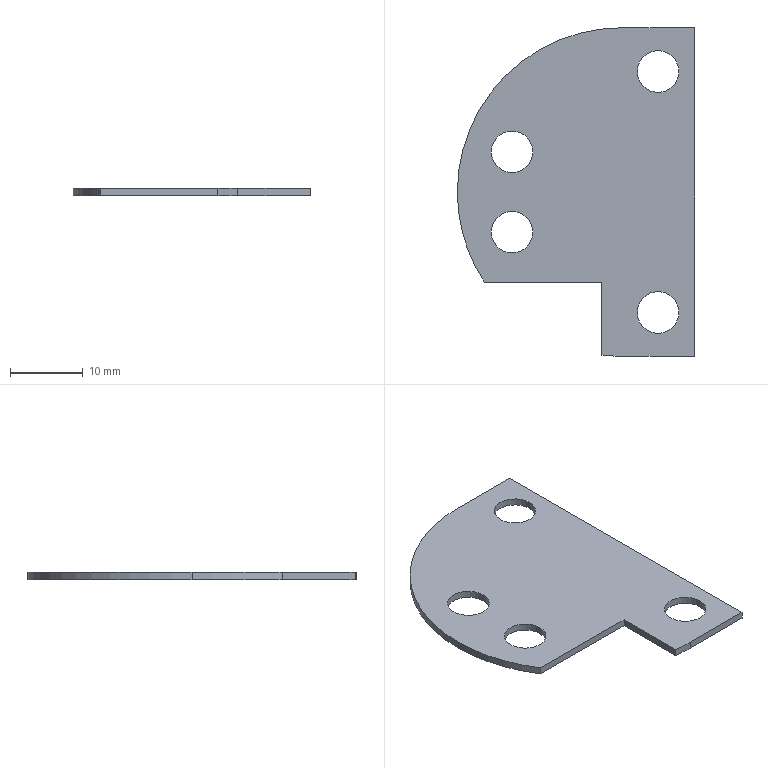Part | SolidWorks | features BaseBody 1, ICE 1 | 1 solid | 18 faces | box 32.5 x 45 x 1 mm | volume 1036 mm3 | cylinder 11 | plane 7 | commonest cylinder face diameters 5.7 x8 45 x3
STEP:
#1=CARTESIAN_POINT('',(-22.85,5.5,1.));
#2=VERTEX_POINT('',#1);
#3=CARTESIAN_POINT('',(-17.15,5.5,1.));
#4=VERTEX_POINT('',#3);
#5=CARTESIAN_POINT('',(-20.,5.5,1.));
#6=DIRECTION('',(0.,0.,1.));
#7=DIRECTION('',(1.,0.,0.));
#8=AXIS2_PLACEMENT_3D('',#5,#6,#7);
#9=CIRCLE('',#8,2.85);
#10=EDGE_CURVE('',#2,#4,#9,.T.);
#11=ORIENTED_EDGE('',*,*,#10,.T.);
#12=CARTESIAN_POINT('',(-17.15,5.5,0.));
#13=VERTEX_POINT('',#12);
#14=CARTESIAN_POINT('',(-17.15,5.5,1.));
#15=DIRECTION('',(0.,0.,-1.));
#16=VECTOR('',#15,1000.);
#17=LINE('',#14,#16);
#18=EDGE_CURVE('',#4,#13,#17,.T.);
#19=ORIENTED_EDGE('',*,*,#18,.T.);
#20=CARTESIAN_POINT('',(-22.85,5.5,0.));
#21=VERTEX_POINT('',#20);
#22=CARTESIAN_POINT('',(-20.,5.5,0.));
#23=DIRECTION('',(0.,0.,1.));
#24=DIRECTION('',(1.,0.,0.));
#25=AXIS2_PLACEMENT_3D('',#22,#23,#24);
#26=CIRCLE('',#25,2.85);
#27=EDGE_CURVE('',#21,#13,#26,.T.);
#28=ORIENTED_EDGE('',*,*,#27,.F.);
#29=CARTESIAN_POINT('',(-22.85,5.5,1.));
#30=DIRECTION('',(0.,0.,-1.));
#31=VECTOR('',#30,1000.);
#32=LINE('',#29,#31);
#33=EDGE_CURVE('',#2,#21,#32,.T.);
#34=ORIENTED_EDGE('',*,*,#33,.F.);
#35=EDGE_LOOP('',(#11,#19,#28,#34));
#36=FACE_OUTER_BOUND('',#35,.T.);
#37=CARTESIAN_POINT('',(-20.,5.5,1.));
#38=DIRECTION('',(0.,0.,-1.));
#39=DIRECTION('',(-1.,0.,0.));
#40=AXIS2_PLACEMENT_3D('',#37,#38,#39);
#41=CYLINDRICAL_SURFACE('',#40,2.85);
#42=ADVANCED_FACE('',(#36),#41,.F.);
#43=CARTESIAN_POINT('',(-22.85,-5.5,1.));
#44=VERTEX_POINT('',#43);
#45=CARTESIAN_POINT('',(-17.15,-5.5,1.));
#46=VERTEX_POINT('',#45);
#47=CARTESIAN_POINT('',(-20.,-5.5,1.));
#48=DIRECTION('',(0.,0.,1.));
#49=DIRECTION('',(1.,0.,0.));
#50=AXIS2_PLACEMENT_3D('',#47,#48,#49);
#51=CIRCLE('',#50,2.85);
#52=EDGE_CURVE('',#44,#46,#51,.T.);
#53=ORIENTED_EDGE('',*,*,#52,.T.);
#54=CARTESIAN_POINT('',(-17.15,-5.5,0.));
#55=VERTEX_POINT('',#54);
#56=CARTESIAN_POINT('',(-17.15,-5.5,1.));
#57=DIRECTION('',(0.,0.,-1.));
#58=VECTOR('',#57,1000.);
#59=LINE('',#56,#58);
#60=EDGE_CURVE('',#46,#55,#59,.T.);
#61=ORIENTED_EDGE('',*,*,#60,.T.);
#62=CARTESIAN_POINT('',(-22.85,-5.5,0.));
#63=VERTEX_POINT('',#62);
#64=CARTESIAN_POINT('',(-20.,-5.5,0.));
#65=DIRECTION('',(0.,0.,1.));
#66=DIRECTION('',(1.,0.,0.));
#67=AXIS2_PLACEMENT_3D('',#64,#65,#66);
#68=CIRCLE('',#67,2.85);
#69=EDGE_CURVE('',#63,#55,#68,.T.);
#70=ORIENTED_EDGE('',*,*,#69,.F.);
#71=CARTESIAN_POINT('',(-22.85,-5.5,1.));
#72=DIRECTION('',(0.,0.,-1.));
#73=VECTOR('',#72,1000.);
#74=LINE('',#71,#73);
#75=EDGE_CURVE('',#44,#63,#74,.T.);
#76=ORIENTED_EDGE('',*,*,#75,.F.);
#77=EDGE_LOOP('',(#53,#61,#70,#76));
#78=FACE_OUTER_BOUND('',#77,.T.);
#79=CARTESIAN_POINT('',(-20.,-5.5,1.));
#80=DIRECTION('',(0.,0.,-1.));
#81=DIRECTION('',(-1.,0.,0.));
#82=AXIS2_PLACEMENT_3D('',#79,#80,#81);
#83=CYLINDRICAL_SURFACE('',#82,2.85);
#84=ADVANCED_FACE('',(#78),#83,.F.);
#85=CARTESIAN_POINT('',(-2.85,-16.5,1.));
#86=VERTEX_POINT('',#85);
#87=CARTESIAN_POINT('',(2.85,-16.5,1.));
#88=VERTEX_POINT('',#87);
#89=CARTESIAN_POINT('',(0.,-16.5,1.));
#90=DIRECTION('',(0.,0.,1.));
#91=DIRECTION('',(1.,0.,0.));
#92=AXIS2_PLACEMENT_3D('',#89,#90,#91);
#93=CIRCLE('',#92,2.85);
#94=EDGE_CURVE('',#86,#88,#93,.T.);
#95=ORIENTED_EDGE('',*,*,#94,.T.);
#96=CARTESIAN_POINT('',(2.85,-16.5,0.));
#97=VERTEX_POINT('',#96);
#98=CARTESIAN_POINT('',(2.85,-16.5,1.));
#99=DIRECTION('',(0.,0.,-1.));
#100=VECTOR('',#99,1000.);
#101=LINE('',#98,#100);
#102=EDGE_CURVE('',#88,#97,#101,.T.);
#103=ORIENTED_EDGE('',*,*,#102,.T.);
#104=CARTESIAN_POINT('',(-2.85,-16.5,0.));
#105=VERTEX_POINT('',#104);
#106=CARTESIAN_POINT('',(0.,-16.5,0.));
#107=DIRECTION('',(0.,0.,1.));
#108=DIRECTION('',(1.,0.,0.));
#109=AXIS2_PLACEMENT_3D('',#106,#107,#108);
#110=CIRCLE('',#109,2.85);
#111=EDGE_CURVE('',#105,#97,#110,.T.);
#112=ORIENTED_EDGE('',*,*,#111,.F.);
#113=CARTESIAN_POINT('',(-2.85,-16.5,1.));
#114=DIRECTION('',(0.,0.,-1.));
#115=VECTOR('',#114,1000.);
#116=LINE('',#113,#115);
#117=EDGE_CURVE('',#86,#105,#116,.T.);
#118=ORIENTED_EDGE('',*,*,#117,.F.);
#119=EDGE_LOOP('',(#95,#103,#112,#118));
#120=FACE_OUTER_BOUND('',#119,.T.);
#121=CARTESIAN_POINT('',(0.,-16.5,1.));
#122=DIRECTION('',(0.,0.,-1.));
#123=DIRECTION('',(-1.,0.,0.));
#124=AXIS2_PLACEMENT_3D('',#121,#122,#123);
#125=CYLINDRICAL_SURFACE('',#124,2.85);
#126=ADVANCED_FACE('',(#120),#125,.F.);
#127=CARTESIAN_POINT('',(-2.85,16.5,1.));
#128=VERTEX_POINT('',#127);
#129=CARTESIAN_POINT('',(2.85,16.5,1.));
#130=VERTEX_POINT('',#129);
#131=CARTESIAN_POINT('',(0.,16.5,1.));
#132=DIRECTION('',(0.,0.,1.));
#133=DIRECTION('',(1.,0.,0.));
#134=AXIS2_PLACEMENT_3D('',#131,#132,#133);
#135=CIRCLE('',#134,2.85);
#136=EDGE_CURVE('',#128,#130,#135,.T.);
#137=ORIENTED_EDGE('',*,*,#136,.T.);
#138=CARTESIAN_POINT('',(2.85,16.5,0.));
#139=VERTEX_POINT('',#138);
#140=CARTESIAN_POINT('',(2.85,16.5,1.));
#141=DIRECTION('',(0.,0.,-1.));
#142=VECTOR('',#141,1000.);
#143=LINE('',#140,#142);
#144=EDGE_CURVE('',#130,#139,#143,.T.);
#145=ORIENTED_EDGE('',*,*,#144,.T.);
#146=CARTESIAN_POINT('',(-2.85,16.5,0.));
#147=VERTEX_POINT('',#146);
#148=CARTESIAN_POINT('',(0.,16.5,0.));
#149=DIRECTION('',(0.,0.,1.));
#150=DIRECTION('',(1.,0.,0.));
#151=AXIS2_PLACEMENT_3D('',#148,#149,#150);
#152=CIRCLE('',#151,2.85);
#153=EDGE_CURVE('',#147,#139,#152,.T.);
#154=ORIENTED_EDGE('',*,*,#153,.F.);
#155=CARTESIAN_POINT('',(-2.85,16.5,1.));
#156=DIRECTION('',(0.,0.,-1.));
#157=VECTOR('',#156,1000.);
#158=LINE('',#155,#157);
#159=EDGE_CURVE('',#128,#147,#158,.T.);
#160=ORIENTED_EDGE('',*,*,#159,.F.);
#161=EDGE_LOOP('',(#137,#145,#154,#160));
#162=FACE_OUTER_BOUND('',#161,.T.);
#163=CARTESIAN_POINT('',(0.,16.5,1.));
#164=DIRECTION('',(0.,0.,-1.));
#165=DIRECTION('',(-1.,0.,0.));
#166=AXIS2_PLACEMENT_3D('',#163,#164,#165);
#167=CYLINDRICAL_SURFACE('',#166,2.85);
#168=ADVANCED_FACE('',(#162),#167,.F.);
#169=CARTESIAN_POINT('',(-27.5,0.,1.));
#170=VERTEX_POINT('',#169);
#171=CARTESIAN_POINT('',(-23.814,-12.34,1.));
#172=VERTEX_POINT('',#171);
#173=CARTESIAN_POINT('',(-5.,0.,1.));
#174=DIRECTION('',(0.,0.,1.));
#175=DIRECTION('',(-1.,0.,0.));
#176=AXIS2_PLACEMENT_3D('',#173,#174,#175);
#177=CIRCLE('',#176,22.5);
#178=EDGE_CURVE('',#170,#172,#177,.T.);
#179=ORIENTED_EDGE('',*,*,#178,.F.);
#180=CARTESIAN_POINT('',(-27.5,0.,0.));
#181=VERTEX_POINT('',#180);
#182=CARTESIAN_POINT('',(-27.5,0.,1.));
#183=DIRECTION('',(0.,0.,-1.));
#184=VECTOR('',#183,1000.);
#185=LINE('',#182,#184);
#186=EDGE_CURVE('',#170,#181,#185,.T.);
#187=ORIENTED_EDGE('',*,*,#186,.T.);
#188=CARTESIAN_POINT('',(-23.814,-12.34,0.));
#189=VERTEX_POINT('',#188);
#190=CARTESIAN_POINT('',(-5.,0.,0.));
#191=DIRECTION('',(0.,0.,1.));
#192=DIRECTION('',(-1.,0.,0.));
#193=AXIS2_PLACEMENT_3D('',#190,#191,#192);
#194=CIRCLE('',#193,22.5);
#195=EDGE_CURVE('',#181,#189,#194,.T.);
#196=ORIENTED_EDGE('',*,*,#195,.T.);
#197=CARTESIAN_POINT('',(-23.814,-12.34,1.));
#198=DIRECTION('',(0.,0.,-1.));
#199=VECTOR('',#198,1000.);
#200=LINE('',#197,#199);
#201=EDGE_CURVE('',#172,#189,#200,.T.);
#202=ORIENTED_EDGE('',*,*,#201,.F.);
#203=EDGE_LOOP('',(#179,#187,#196,#202));
#204=FACE_OUTER_BOUND('',#203,.T.);
#205=CARTESIAN_POINT('',(-5.,0.,1.));
#206=DIRECTION('',(0.,0.,-1.));
#207=DIRECTION('',(-1.,0.,0.));
#208=AXIS2_PLACEMENT_3D('',#205,#206,#207);
#209=CYLINDRICAL_SURFACE('',#208,22.5);
#210=ADVANCED_FACE('',(#204),#209,.T.);
#211=ORIENTED_EDGE('',*,*,#186,.F.);
#212=CARTESIAN_POINT('',(-5.,22.5,1.));
#213=VERTEX_POINT('',#212);
#214=CARTESIAN_POINT('',(-5.,0.,1.));
#215=DIRECTION('',(0.,0.,1.));
#216=DIRECTION('',(-1.,0.,0.));
#217=AXIS2_PLACEMENT_3D('',#214,#215,#216);
#218=CIRCLE('',#217,22.5);
#219=EDGE_CURVE('',#213,#170,#218,.T.);
#220=ORIENTED_EDGE('',*,*,#219,.F.);
#221=CARTESIAN_POINT('',(-5.,22.5,0.));
#222=VERTEX_POINT('',#221);
#223=CARTESIAN_POINT('',(-5.,22.5,1.));
#224=DIRECTION('',(0.,0.,-1.));
#225=VECTOR('',#224,1000.);
#226=LINE('',#223,#225);
#227=EDGE_CURVE('',#213,#222,#226,.T.);
#228=ORIENTED_EDGE('',*,*,#227,.T.);
#229=CARTESIAN_POINT('',(-5.,0.,0.));
#230=DIRECTION('',(0.,0.,1.));
#231=DIRECTION('',(-1.,0.,0.));
#232=AXIS2_PLACEMENT_3D('',#229,#230,#231);
#233=CIRCLE('',#232,22.5);
#234=EDGE_CURVE('',#222,#181,#233,.T.);
#235=ORIENTED_EDGE('',*,*,#234,.T.);
#236=EDGE_LOOP('',(#211,#220,#228,#235));
#237=FACE_OUTER_BOUND('',#236,.T.);
#238=CARTESIAN_POINT('',(-5.,0.,1.));
#239=DIRECTION('',(0.,0.,-1.));
#240=DIRECTION('',(-1.,0.,0.));
#241=AXIS2_PLACEMENT_3D('',#238,#239,#240);
#242=CYLINDRICAL_SURFACE('',#241,22.5);
#243=ADVANCED_FACE('',(#237),#242,.T.);
#244=CARTESIAN_POINT('',(-7.7,-12.34,1.));
#245=VERTEX_POINT('',#244);
#246=CARTESIAN_POINT('',(-7.7,-12.34,1.));
#247=DIRECTION('',(-1.,0.,0.));
#248=VECTOR('',#247,1000.);
#249=LINE('',#246,#248);
#250=EDGE_CURVE('',#245,#172,#249,.T.);
#251=ORIENTED_EDGE('',*,*,#250,.F.);
#252=CARTESIAN_POINT('',(-7.7,-22.337,1.));
#253=VERTEX_POINT('',#252);
#254=CARTESIAN_POINT('',(-7.7,-12.34,1.));
#255=DIRECTION('',(0.,-1.,0.));
#256=VECTOR('',#255,1000.);
#257=LINE('',#254,#256);
#258=EDGE_CURVE('',#245,#253,#257,.T.);
#259=ORIENTED_EDGE('',*,*,#258,.T.);
#260=CARTESIAN_POINT('',(-5.,-22.5,1.));
#261=VERTEX_POINT('',#260);
#262=CARTESIAN_POINT('',(-5.,0.,1.));
#263=DIRECTION('',(0.,0.,1.));
#264=DIRECTION('',(-1.,0.,0.));
#265=AXIS2_PLACEMENT_3D('',#262,#263,#264);
#266=CIRCLE('',#265,22.5);
#267=EDGE_CURVE('',#253,#261,#266,.T.);
#268=ORIENTED_EDGE('',*,*,#267,.T.);
#269=CARTESIAN_POINT('',(5.,-22.5,1.));
#270=VERTEX_POINT('',#269);
#271=CARTESIAN_POINT('',(-5.,-22.5,1.));
#272=DIRECTION('',(1.,0.,0.));
#273=VECTOR('',#272,1000.);
#274=LINE('',#271,#273);
#275=EDGE_CURVE('',#261,#270,#274,.T.);
#276=ORIENTED_EDGE('',*,*,#275,.T.);
#277=CARTESIAN_POINT('',(5.,22.5,1.));
#278=VERTEX_POINT('',#277);
#279=CARTESIAN_POINT('',(5.,-22.5,1.));
#280=DIRECTION('',(0.,1.,0.));
#281=VECTOR('',#280,1000.);
#282=LINE('',#279,#281);
#283=EDGE_CURVE('',#270,#278,#282,.T.);
#284=ORIENTED_EDGE('',*,*,#283,.T.);
#285=CARTESIAN_POINT('',(-5.,22.5,1.));
#286=DIRECTION('',(-1.,0.,0.));
#287=VECTOR('',#286,1000.);
#288=LINE('',#285,#287);
#289=EDGE_CURVE('',#278,#213,#288,.T.);
#290=ORIENTED_EDGE('',*,*,#289,.T.);
#291=ORIENTED_EDGE('',*,*,#219,.T.);
#292=ORIENTED_EDGE('',*,*,#178,.T.);
#293=EDGE_LOOP('',(#251,#259,#268,#276,#284,#290,#291,#292));
#294=FACE_OUTER_BOUND('',#293,.T.);
#295=ORIENTED_EDGE('',*,*,#136,.F.);
#296=CARTESIAN_POINT('',(0.,16.5,1.));
#297=DIRECTION('',(0.,0.,1.));
#298=DIRECTION('',(1.,0.,0.));
#299=AXIS2_PLACEMENT_3D('',#296,#297,#298);
#300=CIRCLE('',#299,2.85);
#301=EDGE_CURVE('',#130,#128,#300,.T.);
#302=ORIENTED_EDGE('',*,*,#301,.F.);
#303=EDGE_LOOP('',(#295,#302));
#304=FACE_BOUND('',#303,.T.);
#305=ORIENTED_EDGE('',*,*,#94,.F.);
#306=CARTESIAN_POINT('',(0.,-16.5,1.));
#307=DIRECTION('',(0.,0.,1.));
#308=DIRECTION('',(1.,0.,0.));
#309=AXIS2_PLACEMENT_3D('',#306,#307,#308);
#310=CIRCLE('',#309,2.85);
#311=EDGE_CURVE('',#88,#86,#310,.T.);
#312=ORIENTED_EDGE('',*,*,#311,.F.);
#313=EDGE_LOOP('',(#305,#312));
#314=FACE_BOUND('',#313,.T.);
#315=ORIENTED_EDGE('',*,*,#52,.F.);
#316=CARTESIAN_POINT('',(-20.,-5.5,1.));
#317=DIRECTION('',(0.,0.,1.));
#318=DIRECTION('',(1.,0.,0.));
#319=AXIS2_PLACEMENT_3D('',#316,#317,#318);
#320=CIRCLE('',#319,2.85);
#321=EDGE_CURVE('',#46,#44,#320,.T.);
#322=ORIENTED_EDGE('',*,*,#321,.F.);
#323=EDGE_LOOP('',(#315,#322));
#324=FACE_BOUND('',#323,.T.);
#325=ORIENTED_EDGE('',*,*,#10,.F.);
#326=CARTESIAN_POINT('',(-20.,5.5,1.));
#327=DIRECTION('',(0.,0.,1.));
#328=DIRECTION('',(1.,0.,0.));
#329=AXIS2_PLACEMENT_3D('',#326,#327,#328);
#330=CIRCLE('',#329,2.85);
#331=EDGE_CURVE('',#4,#2,#330,.T.);
#332=ORIENTED_EDGE('',*,*,#331,.F.);
#333=EDGE_LOOP('',(#325,#332));
#334=FACE_BOUND('',#333,.T.);
#335=CARTESIAN_POINT('',(-5.,0.,1.));
#336=DIRECTION('',(0.,0.,-1.));
#337=DIRECTION('',(-1.,0.,0.));
#338=AXIS2_PLACEMENT_3D('',#335,#336,#337);
#339=PLANE('',#338);
#340=ADVANCED_FACE('',(#294,#304,#314,#324,#334),#339,.F.);
#341=CARTESIAN_POINT('',(-7.7,-12.34,0.));
#342=VERTEX_POINT('',#341);
#343=CARTESIAN_POINT('',(-7.7,-22.337,0.));
#344=VERTEX_POINT('',#343);
#345=CARTESIAN_POINT('',(-7.7,-12.34,0.));
#346=DIRECTION('',(0.,-1.,0.));
#347=VECTOR('',#346,1000.);
#348=LINE('',#345,#347);
#349=EDGE_CURVE('',#342,#344,#348,.T.);
#350=ORIENTED_EDGE('',*,*,#349,.F.);
#351=CARTESIAN_POINT('',(-7.7,-12.34,0.));
#352=DIRECTION('',(-1.,0.,0.));
#353=VECTOR('',#352,1000.);
#354=LINE('',#351,#353);
#355=EDGE_CURVE('',#342,#189,#354,.T.);
#356=ORIENTED_EDGE('',*,*,#355,.T.);
#357=ORIENTED_EDGE('',*,*,#195,.F.);
#358=ORIENTED_EDGE('',*,*,#234,.F.);
#359=CARTESIAN_POINT('',(5.,22.5,0.));
#360=VERTEX_POINT('',#359);
#361=CARTESIAN_POINT('',(-5.,22.5,0.));
#362=DIRECTION('',(-1.,0.,0.));
#363=VECTOR('',#362,1000.);
#364=LINE('',#361,#363);
#365=EDGE_CURVE('',#360,#222,#364,.T.);
#366=ORIENTED_EDGE('',*,*,#365,.F.);
#367=CARTESIAN_POINT('',(5.,-22.5,0.));
#368=VERTEX_POINT('',#367);
#369=CARTESIAN_POINT('',(5.,-22.5,0.));
#370=DIRECTION('',(0.,1.,0.));
#371=VECTOR('',#370,1000.);
#372=LINE('',#369,#371);
#373=EDGE_CURVE('',#368,#360,#372,.T.);
#374=ORIENTED_EDGE('',*,*,#373,.F.);
#375=CARTESIAN_POINT('',(-5.,-22.5,0.));
#376=VERTEX_POINT('',#375);
#377=CARTESIAN_POINT('',(-5.,-22.5,0.));
#378=DIRECTION('',(1.,0.,0.));
#379=VECTOR('',#378,1000.);
#380=LINE('',#377,#379);
#381=EDGE_CURVE('',#376,#368,#380,.T.);
#382=ORIENTED_EDGE('',*,*,#381,.F.);
#383=CARTESIAN_POINT('',(-5.,0.,0.));
#384=DIRECTION('',(0.,0.,1.));
#385=DIRECTION('',(-1.,0.,0.));
#386=AXIS2_PLACEMENT_3D('',#383,#384,#385);
#387=CIRCLE('',#386,22.5);
#388=EDGE_CURVE('',#344,#376,#387,.T.);
#389=ORIENTED_EDGE('',*,*,#388,.F.);
#390=EDGE_LOOP('',(#350,#356,#357,#358,#366,#374,#382,#389));
#391=FACE_OUTER_BOUND('',#390,.T.);
#392=ORIENTED_EDGE('',*,*,#69,.T.);
#393=CARTESIAN_POINT('',(-20.,-5.5,0.));
#394=DIRECTION('',(0.,0.,1.));
#395=DIRECTION('',(1.,0.,0.));
#396=AXIS2_PLACEMENT_3D('',#393,#394,#395);
#397=CIRCLE('',#396,2.85);
#398=EDGE_CURVE('',#55,#63,#397,.T.);
#399=ORIENTED_EDGE('',*,*,#398,.T.);
#400=EDGE_LOOP('',(#392,#399));
#401=FACE_BOUND('',#400,.T.);
#402=ORIENTED_EDGE('',*,*,#153,.T.);
#403=CARTESIAN_POINT('',(0.,16.5,0.));
#404=DIRECTION('',(0.,0.,1.));
#405=DIRECTION('',(1.,0.,0.));
#406=AXIS2_PLACEMENT_3D('',#403,#404,#405);
#407=CIRCLE('',#406,2.85);
#408=EDGE_CURVE('',#139,#147,#407,.T.);
#409=ORIENTED_EDGE('',*,*,#408,.T.);
#410=EDGE_LOOP('',(#402,#409));
#411=FACE_BOUND('',#410,.T.);
#412=ORIENTED_EDGE('',*,*,#111,.T.);
#413=CARTESIAN_POINT('',(0.,-16.5,0.));
#414=DIRECTION('',(0.,0.,1.));
#415=DIRECTION('',(1.,0.,0.));
#416=AXIS2_PLACEMENT_3D('',#413,#414,#415);
#417=CIRCLE('',#416,2.85);
#418=EDGE_CURVE('',#97,#105,#417,.T.);
#419=ORIENTED_EDGE('',*,*,#418,.T.);
#420=EDGE_LOOP('',(#412,#419));
#421=FACE_BOUND('',#420,.T.);
#422=ORIENTED_EDGE('',*,*,#27,.T.);
#423=CARTESIAN_POINT('',(-20.,5.5,0.));
#424=DIRECTION('',(0.,0.,1.));
#425=DIRECTION('',(1.,0.,0.));
#426=AXIS2_PLACEMENT_3D('',#423,#424,#425);
#427=CIRCLE('',#426,2.85);
#428=EDGE_CURVE('',#13,#21,#427,.T.);
#429=ORIENTED_EDGE('',*,*,#428,.T.);
#430=EDGE_LOOP('',(#422,#429));
#431=FACE_BOUND('',#430,.T.);
#432=CARTESIAN_POINT('',(-5.,0.,0.));
#433=DIRECTION('',(0.,0.,-1.));
#434=DIRECTION('',(-1.,0.,0.));
#435=AXIS2_PLACEMENT_3D('',#432,#433,#434);
#436=PLANE('',#435);
#437=ADVANCED_FACE('',(#391,#401,#411,#421,#431),#436,.T.);
#438=ORIENTED_EDGE('',*,*,#373,.T.);
#439=CARTESIAN_POINT('',(5.,22.5,1.));
#440=DIRECTION('',(0.,0.,-1.));
#441=VECTOR('',#440,1000.);
#442=LINE('',#439,#441);
#443=EDGE_CURVE('',#278,#360,#442,.T.);
#444=ORIENTED_EDGE('',*,*,#443,.F.);
#445=ORIENTED_EDGE('',*,*,#283,.F.);
#446=CARTESIAN_POINT('',(5.,-22.5,1.));
#447=DIRECTION('',(0.,0.,-1.));
#448=VECTOR('',#447,1000.);
#449=LINE('',#446,#448);
#450=EDGE_CURVE('',#270,#368,#449,.T.);
#451=ORIENTED_EDGE('',*,*,#450,.T.);
#452=EDGE_LOOP('',(#438,#444,#445,#451));
#453=FACE_OUTER_BOUND('',#452,.T.);
#454=CARTESIAN_POINT('',(5.,-22.5,1.));
#455=DIRECTION('',(-1.,0.,0.));
#456=DIRECTION('',(0.,-1.,0.));
#457=AXIS2_PLACEMENT_3D('',#454,#455,#456);
#458=PLANE('',#457);
#459=ADVANCED_FACE('',(#453),#458,.F.);
#460=ORIENTED_EDGE('',*,*,#365,.T.);
#461=ORIENTED_EDGE('',*,*,#227,.F.);
#462=ORIENTED_EDGE('',*,*,#289,.F.);
#463=ORIENTED_EDGE('',*,*,#443,.T.);
#464=EDGE_LOOP('',(#460,#461,#462,#463));
#465=FACE_OUTER_BOUND('',#464,.T.);
#466=CARTESIAN_POINT('',(-5.,22.5,1.));
#467=DIRECTION('',(0.,-1.,0.));
#468=DIRECTION('',(0.,0.,-1.));
#469=AXIS2_PLACEMENT_3D('',#466,#467,#468);
#470=PLANE('',#469);
#471=ADVANCED_FACE('',(#465),#470,.F.);
#472=ORIENTED_EDGE('',*,*,#267,.F.);
#473=CARTESIAN_POINT('',(-7.7,-22.337,1.));
#474=DIRECTION('',(0.,0.,-1.));
#475=VECTOR('',#474,1000.);
#476=LINE('',#473,#475);
#477=EDGE_CURVE('',#253,#344,#476,.T.);
#478=ORIENTED_EDGE('',*,*,#477,.T.);
#479=ORIENTED_EDGE('',*,*,#388,.T.);
#480=CARTESIAN_POINT('',(-5.,-22.5,1.));
#481=DIRECTION('',(0.,0.,-1.));
#482=VECTOR('',#481,1000.);
#483=LINE('',#480,#482);
#484=EDGE_CURVE('',#261,#376,#483,.T.);
#485=ORIENTED_EDGE('',*,*,#484,.F.);
#486=EDGE_LOOP('',(#472,#478,#479,#485));
#487=FACE_OUTER_BOUND('',#486,.T.);
#488=CARTESIAN_POINT('',(-5.,0.,1.));
#489=DIRECTION('',(0.,0.,-1.));
#490=DIRECTION('',(-1.,0.,0.));
#491=AXIS2_PLACEMENT_3D('',#488,#489,#490);
#492=CYLINDRICAL_SURFACE('',#491,22.5);
#493=ADVANCED_FACE('',(#487),#492,.T.);
#494=ORIENTED_EDGE('',*,*,#381,.T.);
#495=ORIENTED_EDGE('',*,*,#450,.F.);
#496=ORIENTED_EDGE('',*,*,#275,.F.);
#497=ORIENTED_EDGE('',*,*,#484,.T.);
#498=EDGE_LOOP('',(#494,#495,#496,#497));
#499=FACE_OUTER_BOUND('',#498,.T.);
#500=CARTESIAN_POINT('',(-5.,-22.5,1.));
#501=DIRECTION('',(0.,1.,0.));
#502=DIRECTION('',(0.,0.,1.));
#503=AXIS2_PLACEMENT_3D('',#500,#501,#502);
#504=PLANE('',#503);
#505=ADVANCED_FACE('',(#499),#504,.F.);
#506=ORIENTED_EDGE('',*,*,#144,.F.);
#507=ORIENTED_EDGE('',*,*,#301,.T.);
#508=ORIENTED_EDGE('',*,*,#159,.T.);
#509=ORIENTED_EDGE('',*,*,#408,.F.);
#510=EDGE_LOOP('',(#506,#507,#508,#509));
#511=FACE_OUTER_BOUND('',#510,.T.);
#512=CARTESIAN_POINT('',(0.,16.5,1.));
#513=DIRECTION('',(0.,0.,-1.));
#514=DIRECTION('',(-1.,0.,0.));
#515=AXIS2_PLACEMENT_3D('',#512,#513,#514);
#516=CYLINDRICAL_SURFACE('',#515,2.85);
#517=ADVANCED_FACE('',(#511),#516,.F.);
#518=ORIENTED_EDGE('',*,*,#102,.F.);
#519=ORIENTED_EDGE('',*,*,#311,.T.);
#520=ORIENTED_EDGE('',*,*,#117,.T.);
#521=ORIENTED_EDGE('',*,*,#418,.F.);
#522=EDGE_LOOP('',(#518,#519,#520,#521));
#523=FACE_OUTER_BOUND('',#522,.T.);
#524=CARTESIAN_POINT('',(0.,-16.5,1.));
#525=DIRECTION('',(0.,0.,-1.));
#526=DIRECTION('',(-1.,0.,0.));
#527=AXIS2_PLACEMENT_3D('',#524,#525,#526);
#528=CYLINDRICAL_SURFACE('',#527,2.85);
#529=ADVANCED_FACE('',(#523),#528,.F.);
#530=ORIENTED_EDGE('',*,*,#60,.F.);
#531=ORIENTED_EDGE('',*,*,#321,.T.);
#532=ORIENTED_EDGE('',*,*,#75,.T.);
#533=ORIENTED_EDGE('',*,*,#398,.F.);
#534=EDGE_LOOP('',(#530,#531,#532,#533));
#535=FACE_OUTER_BOUND('',#534,.T.);
#536=CARTESIAN_POINT('',(-20.,-5.5,1.));
#537=DIRECTION('',(0.,0.,-1.));
#538=DIRECTION('',(-1.,0.,0.));
#539=AXIS2_PLACEMENT_3D('',#536,#537,#538);
#540=CYLINDRICAL_SURFACE('',#539,2.85);
#541=ADVANCED_FACE('',(#535),#540,.F.);
#542=ORIENTED_EDGE('',*,*,#18,.F.);
#543=ORIENTED_EDGE('',*,*,#331,.T.);
#544=ORIENTED_EDGE('',*,*,#33,.T.);
#545=ORIENTED_EDGE('',*,*,#428,.F.);
#546=EDGE_LOOP('',(#542,#543,#544,#545));
#547=FACE_OUTER_BOUND('',#546,.T.);
#548=CARTESIAN_POINT('',(-20.,5.5,1.));
#549=DIRECTION('',(0.,0.,-1.));
#550=DIRECTION('',(-1.,0.,0.));
#551=AXIS2_PLACEMENT_3D('',#548,#549,#550);
#552=CYLINDRICAL_SURFACE('',#551,2.85);
#553=ADVANCED_FACE('',(#547),#552,.F.);
#554=ORIENTED_EDGE('',*,*,#349,.T.);
#555=ORIENTED_EDGE('',*,*,#477,.F.);
#556=ORIENTED_EDGE('',*,*,#258,.F.);
#557=CARTESIAN_POINT('',(-7.7,-12.34,1.));
#558=DIRECTION('',(0.,0.,-1.));
#559=VECTOR('',#558,1000.);
#560=LINE('',#557,#559);
#561=EDGE_CURVE('',#245,#342,#560,.T.);
#562=ORIENTED_EDGE('',*,*,#561,.T.);
#563=EDGE_LOOP('',(#554,#555,#556,#562));
#564=FACE_OUTER_BOUND('',#563,.T.);
#565=CARTESIAN_POINT('',(-7.7,-12.34,1.));
#566=DIRECTION('',(1.,0.,0.));
#567=DIRECTION('',(0.,1.,0.));
#568=AXIS2_PLACEMENT_3D('',#565,#566,#567);
#569=PLANE('',#568);
#570=ADVANCED_FACE('',(#564),#569,.F.);
#571=ORIENTED_EDGE('',*,*,#355,.F.);
#572=ORIENTED_EDGE('',*,*,#561,.F.);
#573=ORIENTED_EDGE('',*,*,#250,.T.);
#574=ORIENTED_EDGE('',*,*,#201,.T.);
#575=EDGE_LOOP('',(#571,#572,#573,#574));
#576=FACE_OUTER_BOUND('',#575,.T.);
#577=CARTESIAN_POINT('',(-7.7,-12.34,1.));
#578=DIRECTION('',(0.,-1.,0.));
#579=DIRECTION('',(0.,0.,-1.));
#580=AXIS2_PLACEMENT_3D('',#577,#578,#579);
#581=PLANE('',#580);
#582=ADVANCED_FACE('',(#576),#581,.T.);
#583=CLOSED_SHELL('',(#42,#84,#126,#168,#210,#243,#340,#437,#459,#471,#493,#505,#517,#529,#541,#553,#570,#582));
#584=MANIFOLD_SOLID_BREP('',#583);
#585=CARTESIAN_POINT('',(0.,0.,0.));
#586=DIRECTION('',(0.,0.,1.));
#587=DIRECTION('',(1.,0.,0.));
#588=AXIS2_PLACEMENT_3D('',#585,#586,#587);
#589=(LENGTH_UNIT()NAMED_UNIT(*)SI_UNIT(.MILLI.,.METRE.));
#590=UNCERTAINTY_MEASURE_WITH_UNIT(LENGTH_MEASURE(0.00001),#589,'','');
#591=(NAMED_UNIT(*)PLANE_ANGLE_UNIT()SI_UNIT($,.RADIAN.));
#592=(NAMED_UNIT(*)SI_UNIT($,.STERADIAN.)SOLID_ANGLE_UNIT());
#593=(GEOMETRIC_REPRESENTATION_CONTEXT(3)GLOBAL_UNCERTAINTY_ASSIGNED_CONTEXT((#590))GLOBAL_UNIT_ASSIGNED_CONTEXT((#589,#591,#592))REPRESENTATION_CONTEXT('',''));
#594=ADVANCED_BREP_SHAPE_REPRESENTATION('',(#584,#588),#593);